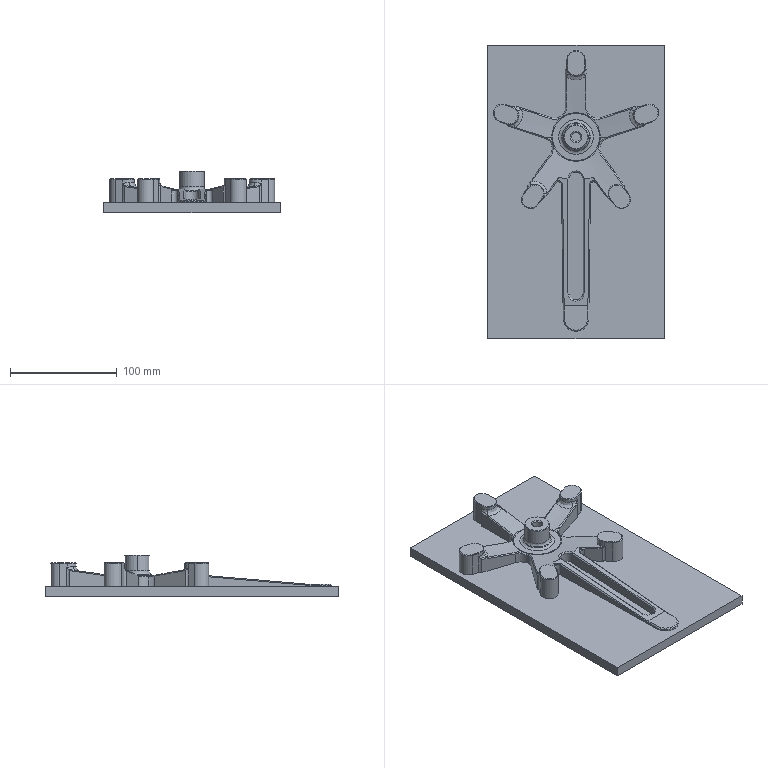CAM job | NX | 3-axis milling | part box 165 x 275 x 39 mm | stock box 165 x 275 x 39 mm
Tools:
number,name,description,diameter,corner_radius,flute_length,length,flutes
0,D12,Milling Tool-5 Parameters,12.0,0.0,50.0,75.0,2
0,D6R3,Milling Tool-Ball Mill,6.0,3.0,50.0,75.0,2
0,D6,Milling Tool-5 Parameters,6.0,0.0,50.0,75.0,2
Operations:
program,operation,operation_type,tool,method,geometry_group,spindle_rpm,surface_speed,feed_per_tooth,feed_cut,feed_plunge,cut_length_mm,path_length_mm,cut_time_min,machine_time_min
NC_PROGRAM,CAVITY_MILL,CavityMilling,D12,METHOD,WORKPIECE,0.0,0.0,0.0,250.0,100.0,463944.851,469588.948,1855.779,1856.344
NC_PROGRAM,CORNER_ROUGH,CavityMilling,D6,METHOD,WORKPIECE,0.0,0.0,0.0,250.0,100.0,6945.557,9443.391,27.782,28.032
NC_PROGRAM,ZLEVEL_PROFILE,ZLevelMilling,D6,METHOD,WORKPIECE,0.0,0.0,0.0,250.0,100.0,370085.273,372657.678,1480.341,1480.598
NC_PROGRAM,FACE_MILLING,FaceMilling,D6,METHOD,WORKPIECE,0.0,0.0,0.0,250.0,100.0,10277.361,11306.953,41.109,41.212
NC_PROGRAM,CONTOUR_AREA,SurfaceContour,D6R3,METHOD,WORKPIECE,0.0,0.0,0.0,250.0,100.0,18546.593,19177.65,74.186,74.249